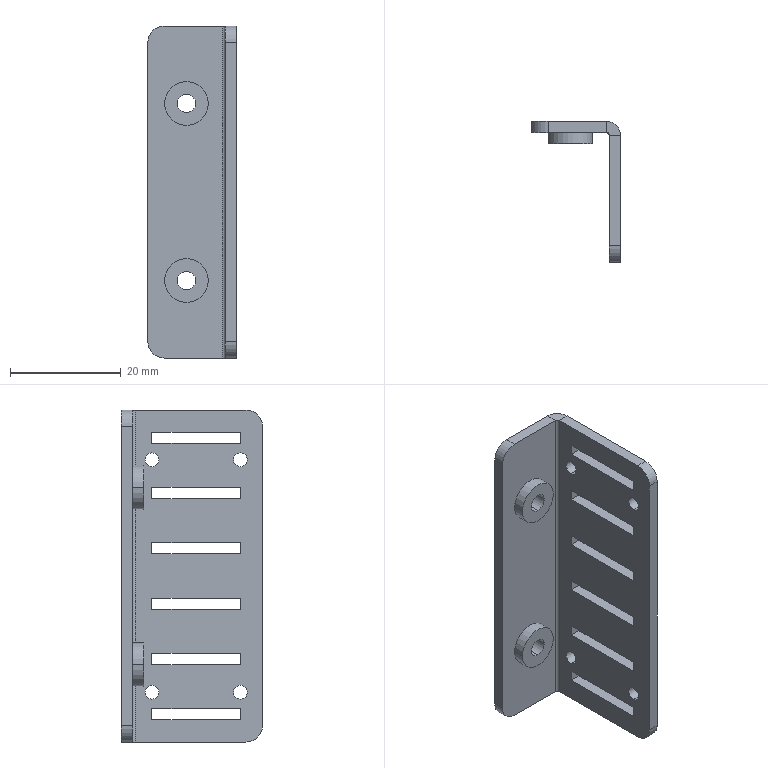Part | SolidWorks | features BaseBody 1 | 1 solid | 60 faces | box 16 x 25.5 x 60 mm | volume 4352 mm3 | plane 38 | cylinder 22 | commonest cylinder face diameters 2.5 x8 3.3 x4 6 x4 7.9 x4 1 x1 5 x1